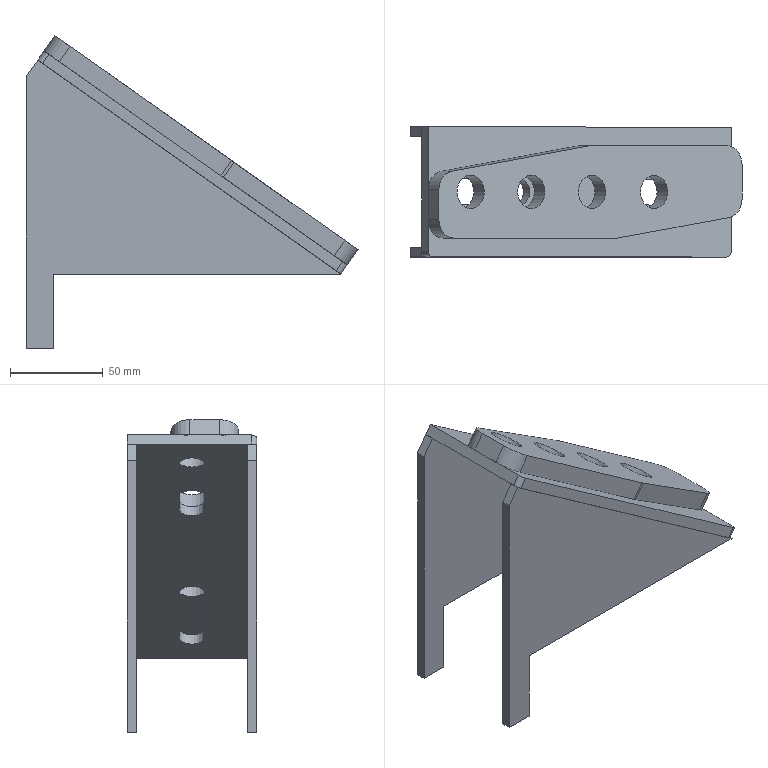Part | STEP file | tensioning conveyor mechanism lower bracket right | 4 solids | 50 faces | box 178.949 x 70 x 168.419 mm | volume 258890 mm3 | plane 34 | cylinder 16 | commonest cylinder face diameters 20 x6 14 x4 18 x4 6 x2